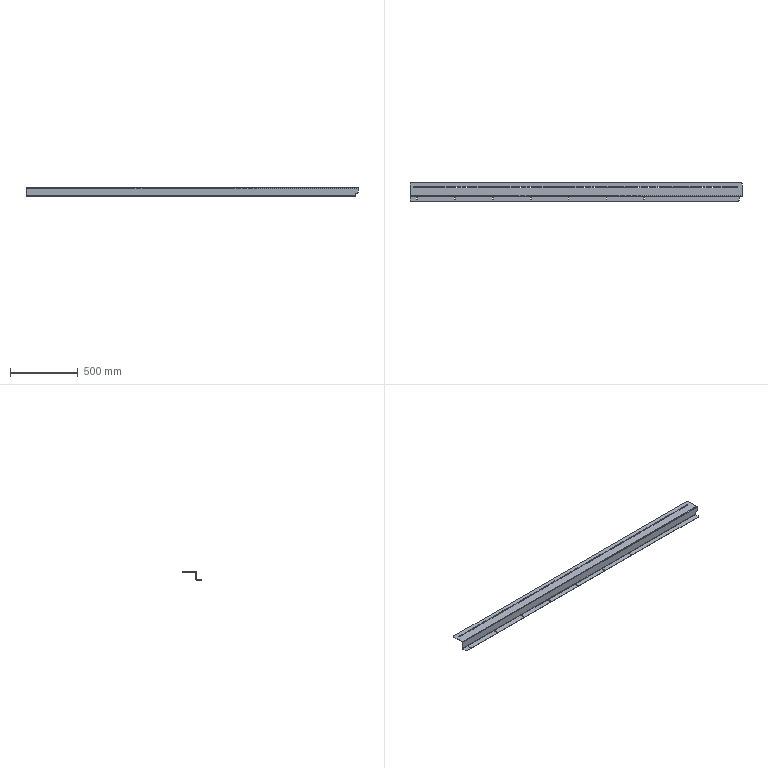Part | SolidWorks | features BaseBody 1 | 1 solid | 149 faces | box 2450 x 138 x 63 mm | volume 924443 mm3 | cylinder 84 | plane 65 | commonest cylinder face diameters 8 x62 6.6 x14 20 x6 4 x2